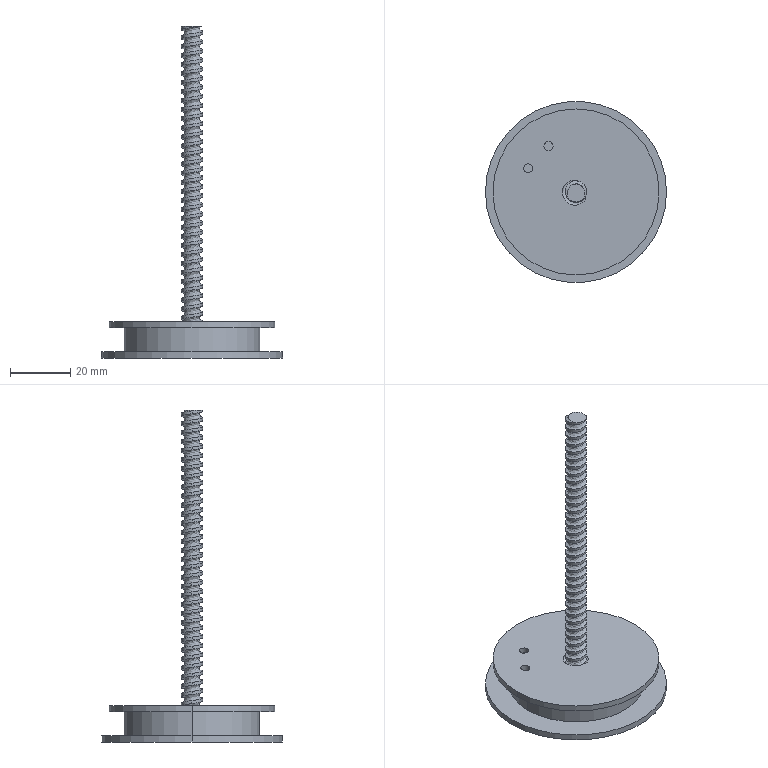Part | SolidWorks | features ICE 3, Cut 2, Extrusion 1, Helix 1, SweepCut 1 | 1 solid | 91 faces | box 60 x 60 x 110.002 mm | volume 25433 mm3 | cylinder 80 | plane 9 | spline 2 | commonest cylinder face diameters 7 x70 3 x4 45 x2 55 x2 60 x2